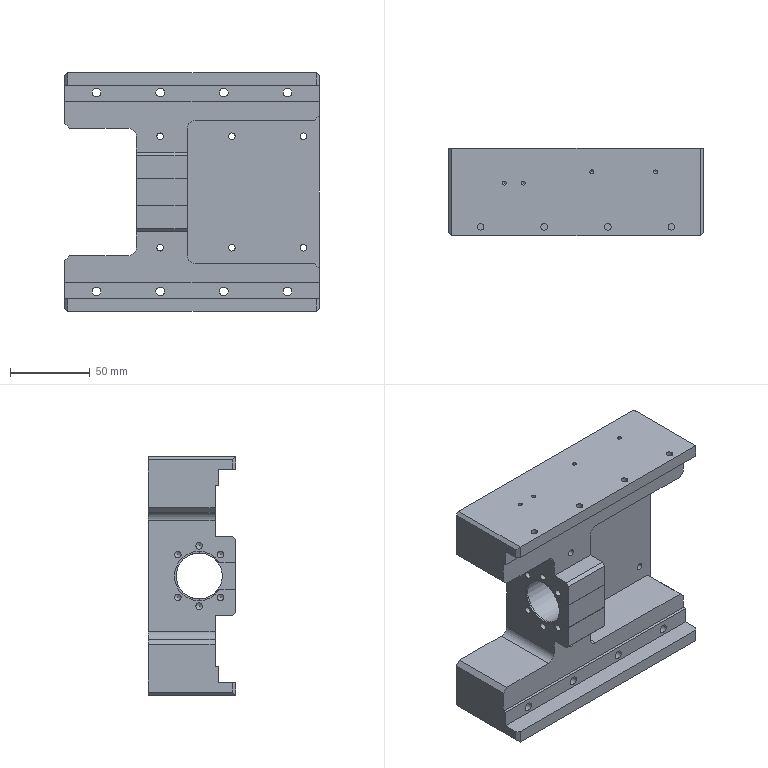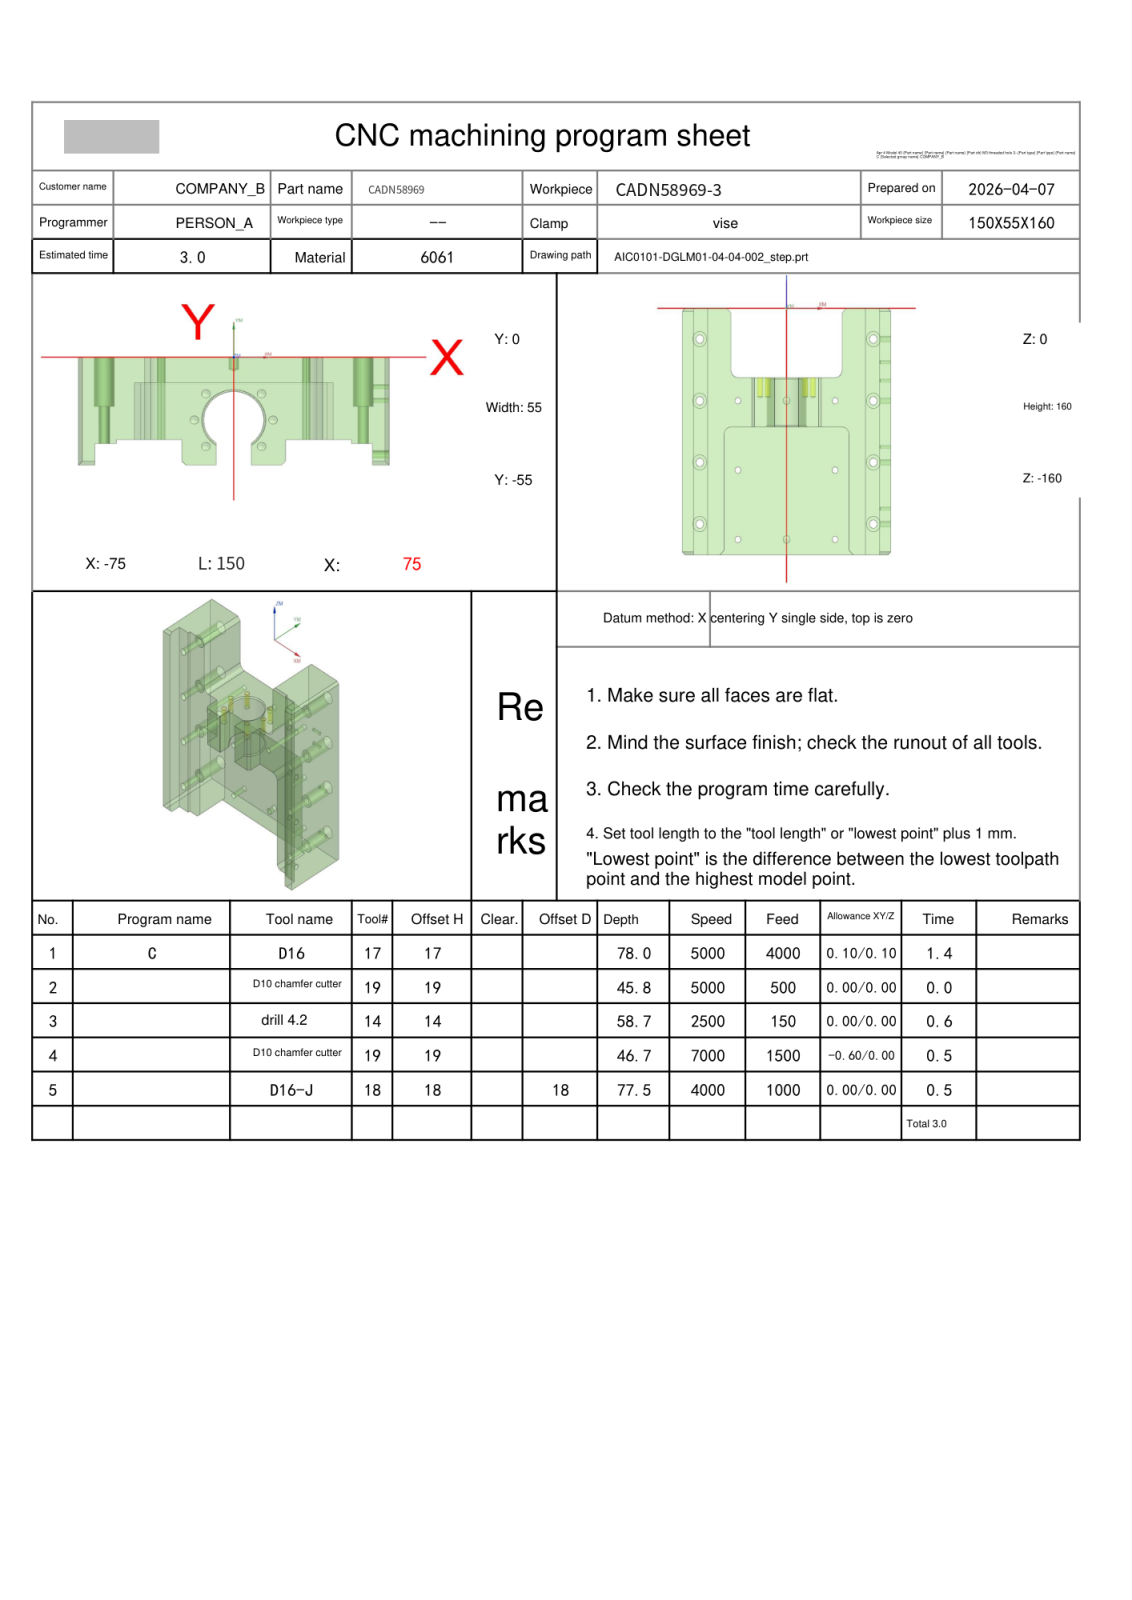NC program | NX | posted by the shop | part box 160 x 55 x 150 mm
Whole program:
%
O0001
(Machine time: 3.92 MIN)
(===Total Tool:4===)
(T17=D16    D=16.  R=0.   D-  H17 Z=-78.  )
(T19=D10 chamfer cutter D=10. R=0. D-H19 Z=-46.7 )
(T14=drill 4.2 D=4.2 DR_a=118 D-H14 Z=-58.66)
(T18=D16-J  D=16.  R=0.   D18 H18 Z=-77.5 )
G80 G90 G17 G49 G40
G91 G28 Z0
M01
N1 T17 M06
(D16  D=16. R=0. H=17 ce=0.10 di=0.10)
G00 G90 G54 X.4 Y-68.796 M03 S5000
G43 H17 Z20.
M08
Z-45.6
G01 Y-54.8 F4000.
Y-44.285
G02 X3.874 Y-37.538 I8.289 J-.001
G03 X6.759 Y-32. I-3.874 J5.538
X0.0 Y-25.241 I-6.759 J0.0
X-6.759 Y-32. I0.0 J-6.759
X-3.908 Y-37.514 I6.759 J0.0
G02 X-.4 Y-44.285 I-4.781 J-6.771
G01 Y-54.8
Y-68.796
G00 Z-46.2
G01 Y-54.8
Y-43.747
G03 X-3.752 Y-37.185 I-8.1 J0.0
G02 X-6.4 Y-32. I3.752 J5.185
X0.0 Y-25.6 I6.4 J0.0
X6.4 Y-32. I0.0 J-6.4
X3.752 Y-37.185 I-6.4 J0.0
G03 X.4 Y-43.747 I4.748 J-6.562
G01 Y-54.8
Y-68.796
G00 Z-46.8
G01 Y-54.8
Y-43.747
G02 X3.752 Y-37.185 I8.1 J0.0
G03 X6.4 Y-32. I-3.752 J5.185
X0.0 Y-25.6 I-6.4 J0.0
X-6.4 Y-32. I0.0 J-6.4
X-3.752 Y-37.185 I6.4 J0.0
G02 X-.4 Y-43.747 I-4.748 J-6.562
G01 Y-54.8
Y-68.796
G00 Z-47.4
G01 Y-54.8
Y-43.747
G03 X-3.752 Y-37.185 I-8.1 J0.0
G02 X-6.4 Y-32. I3.752 J5.185
X0.0 Y-25.6 I6.4 J0.0
X6.4 Y-32. I0.0 J-6.4
X3.752 Y-37.185 I-6.4 J0.0
G03 X.4 Y-43.747 I4.748 J-6.562
G01 Y-54.8
Y-68.796
G00 Z-48.
G01 Y-54.8
Y-43.747
G02 X3.752 Y-37.185 I8.1 J0.0
G03 X6.4 Y-32. I-3.752 J5.185
X0.0 Y-25.6 I-6.4 J0.0
X-6.4 Y-32. I0.0 J-6.4
X-3.752 Y-37.185 I6.4 J0.0
G02 X-.4 Y-43.747 I-4.748 J-6.562
G01 Y-54.8
Y-68.796
G00 Z-48.6
G01 Y-54.8
Y-43.747
G03 X-3.752 Y-37.185 I-8.1 J0.0
G02 X-6.4 Y-32. I3.752 J5.185
X0.0 Y-25.6 I6.4 J0.0
X6.4 Y-32. I0.0 J-6.4
X3.752 Y-37.185 I-6.4 J0.0
G03 X.4 Y-43.747 I4.748 J-6.562
G01 Y-54.8
Y-68.796
G00 Z-49.2
G01 Y-54.8
Y-43.747
G02 X3.752 Y-37.185 I8.1 J0.0
G03 X6.4 Y-32. I-3.752 J5.185
X0.0 Y-25.6 I-6.4 J0.0
X-6.4 Y-32. I0.0 J-6.4
X-3.752 Y-37.185 I6.4 J0.0
G02 X-.4 Y-43.747 I-4.748 J-6.562
G01 Y-54.8
Y-68.796
G00 Z-49.8
G01 Y-54.8
Y-43.747
G03 X-3.752 Y-37.185 I-8.1 J0.0
G02 X-6.4 Y-32. I3.752 J5.185
X0.0 Y-25.6 I6.4 J0.0
X6.4 Y-32. I0.0 J-6.4
X3.752 Y-37.185 I-6.4 J0.0
G03 X.4 Y-43.747 I4.748 J-6.562
G01 Y-54.8
Y-68.796
G00 Z-50.4
G01 Y-54.8
Y-43.747
G02 X3.752 Y-37.185 I8.1 J0.0
G03 X6.4 Y-32. I-3.752 J5.185
X0.0 Y-25.6 I-6.4 J0.0
X-6.4 Y-32. I0.0 J-6.4
X-3.752 Y-37.185 I6.4 J0.0
G02 X-.4 Y-43.747 I-4.748 J-6.562
G01 Y-54.8
Y-68.796
G00 Z-51.
G01 Y-54.8
Y-43.747
G03 X-3.752 Y-37.185 I-8.1 J0.0
G02 X-6.4 Y-32. I3.752 J5.185
X0.0 Y-25.6 I6.4 J0.0
X6.4 Y-32. I0.0 J-6.4
X3.752 Y-37.185 I-6.4 J0.0
G03 X.4 Y-43.747 I4.748 J-6.562
G01 Y-54.8
Y-68.796
G00 Z-51.6
G01 Y-54.8
Y-43.747
G02 X3.752 Y-37.185 I8.1 J0.0
G03 X6.4 Y-32. I-3.752 J5.185
X0.0 Y-25.6 I-6.4 J0.0
X-6.4 Y-32. I0.0 J-6.4
X-3.752 Y-37.185 I6.4 J0.0
G02 X-.4 Y-43.747 I-4.748 J-6.562
G01 Y-54.8
Y-68.796
G00 Z-52.2
G01 Y-54.8
Y-43.747
G03 X-3.752 Y-37.185 I-8.1 J0.0
G02 X-6.4 Y-32. I3.752 J5.185
X0.0 Y-25.6 I6.4 J0.0
X6.4 Y-32. I0.0 J-6.4
X3.752 Y-37.185 I-6.4 J0.0
G03 X.4 Y-43.747 I4.748 J-6.562
G01 Y-54.8
Y-68.796
G00 Z-52.8
G01 Y-54.8
Y-43.747
G02 X3.752 Y-37.185 I8.1 J0.0
G03 X6.4 Y-32. I-3.752 J5.185
X0.0 Y-25.6 I-6.4 J0.0
X-6.4 Y-32. I0.0 J-6.4
X-3.752 Y-37.185 I6.4 J0.0
G02 X-.4 Y-43.747 I-4.748 J-6.562
G01 Y-54.8
Y-68.796
G00 Z-53.4
G01 Y-54.8
Y-43.747
G03 X-3.752 Y-37.185 I-8.1 J0.0
G02 X-6.4 Y-32. I3.752 J5.185
X0.0 Y-25.6 I6.4 J0.0
X6.4 Y-32. I0.0 J-6.4
X3.752 Y-37.185 I-6.4 J0.0
G03 X.4 Y-43.747 I4.748 J-6.562
G01 Y-54.8
Y-68.796
G00 Z-54.
G01 Y-54.8
Y-43.747
G02 X3.752 Y-37.185 I8.1 J0.0
G03 X6.4 Y-32. I-3.752 J5.185
X0.0 Y-25.6 I-6.4 J0.0
X-6.4 Y-32. I0.0 J-6.4
X-3.752 Y-37.185 I6.4 J0.0
G02 X-.4 Y-43.747 I-4.748 J-6.562
G01 Y-54.8
Y-68.796
G00 Z-54.6
G01 Y-54.8
Y-43.747
G03 X-3.752 Y-37.185 I-8.1 J0.0
G02 X-6.4 Y-32. I3.752 J5.185
X0.0 Y-25.6 I6.4 J0.0
X6.4 Y-32. I0.0 J-6.4
X3.752 Y-37.185 I-6.4 J0.0
G03 X.4 Y-43.747 I4.748 J-6.562
G01 Y-54.8
Y-68.796
G00 Z-55.2
G01 Y-54.8
Y-43.747
G02 X3.752 Y-37.185 I8.1 J0.0
G03 X6.4 Y-32. I-3.752 J5.185
X0.0 Y-25.6 I-6.4 J0.0
X-6.4 Y-32. I0.0 J-6.4
X-3.752 Y-37.185 I6.4 J0.0
G02 X-.4 Y-43.747 I-4.748 J-6.562
G01 Y-54.8
Y-68.796
G00 Z-55.8
G01 Y-54.8
Y-43.747
G03 X-3.752 Y-37.185 I-8.1 J0.0
G02 X-6.4 Y-32. I3.752 J5.185
X0.0 Y-25.6 I6.4 J0.0
X6.4 Y-32. I0.0 J-6.4
X3.752 Y-37.185 I-6.4 J0.0
G03 X.4 Y-43.747 I4.748 J-6.562
G01 Y-54.8
Y-68.796
G00 Z-56.4
G01 Y-54.8
Y-43.747
G02 X3.752 Y-37.185 I8.1 J0.0
G03 X6.4 Y-32. I-3.752 J5.185
X0.0 Y-25.6 I-6.4 J0.0
X-6.4 Y-32. I0.0 J-6.4
X-3.752 Y-37.185 I6.4 J0.0
G02 X-.4 Y-43.747 I-4.748 J-6.562
G01 Y-54.8
Y-68.796
G00 Z-57.
G01 Y-54.8
Y-43.747
G03 X-3.752 Y-37.185 I-8.1 J0.0
G02 X-6.4 Y-32. I3.752 J5.185
X0.0 Y-25.6 I6.4 J0.0
X6.4 Y-32. I0.0 J-6.4
X3.752 Y-37.185 I-6.4 J0.0
G03 X.4 Y-43.747 I4.748 J-6.562
G01 Y-54.8
Y-68.796
G00 Z-57.6
G01 Y-54.8
Y-43.747
G02 X3.752 Y-37.185 I8.1 J0.0
G03 X6.4 Y-32. I-3.752 J5.185
X0.0 Y-25.6 I-6.4 J0.0
X-6.4 Y-32. I0.0 J-6.4
X-3.752 Y-37.185 I6.4 J0.0
G02 X-.4 Y-43.747 I-4.748 J-6.562
G01 Y-54.8
Y-68.796
G00 Z-58.2
G01 Y-54.8
Y-43.747
G03 X-3.752 Y-37.185 I-8.1 J0.0
G02 X-6.4 Y-32. I3.752 J5.185
X0.0 Y-25.6 I6.4 J0.0
X6.4 Y-32. I0.0 J-6.4
X3.752 Y-37.185 I-6.4 J0.0
G03 X.4 Y-43.747 I4.748 J-6.562
G01 Y-54.8
Y-68.796
G00 Z-58.8
G01 Y-54.8
Y-43.747
G02 X3.752 Y-37.185 I8.1 J0.0
G03 X6.4 Y-32. I-3.752 J5.185
X0.0 Y-25.6 I-6.4 J0.0
X-6.4 Y-32. I0.0 J-6.4
X-3.752 Y-37.185 I6.4 J0.0
G02 X-.4 Y-43.747 I-4.748 J-6.562
G01 Y-54.8
Y-68.796
G00 Z-59.4
G01 Y-54.8
Y-43.747
G03 X-3.752 Y-37.185 I-8.1 J0.0
G02 X-6.4 Y-32. I3.752 J5.185
X0.0 Y-25.6 I6.4 J0.0
X6.4 Y-32. I0.0 J-6.4
X3.752 Y-37.185 I-6.4 J0.0
G03 X.4 Y-43.747 I4.748 J-6.562
G01 Y-54.8
Y-68.796
G00 Z-60.
G01 Y-54.8
Y-43.747
G02 X3.752 Y-37.185 I8.1 J0.0
G03 X6.4 Y-32. I-3.752 J5.185
X0.0 Y-25.6 I-6.4 J0.0
X-6.4 Y-32. I0.0 J-6.4
X-3.752 Y-37.185 I6.4 J0.0
G02 X-.4 Y-43.747 I-4.748 J-6.562
G01 Y-54.8
Y-68.796
G00 Z-60.6
G01 Y-54.8
Y-43.747
G03 X-3.752 Y-37.185 I-8.1 J0.0
G02 X-6.4 Y-32. I3.752 J5.185
X0.0 Y-25.6 I6.4 J0.0
X6.4 Y-32. I0.0 J-6.4
X3.752 Y-37.185 I-6.4 J0.0
G03 X.4 Y-43.747 I4.748 J-6.562
G01 Y-54.8
Y-68.796
G00 Z-61.2
G01 Y-54.8
Y-43.747
G02 X3.752 Y-37.185 I8.1 J0.0
G03 X6.4 Y-32. I-3.752 J5.185
X0.0 Y-25.6 I-6.4 J0.0
X-6.4 Y-32. I0.0 J-6.4
X-3.752 Y-37.185 I6.4 J0.0
G02 X-.4 Y-43.747 I-4.748 J-6.562
G01 Y-54.8
Y-68.796
G00 Z-61.8
G01 Y-54.8
Y-43.747
G03 X-3.752 Y-37.185 I-8.1 J0.0
G02 X-6.4 Y-32. I3.752 J5.185
X0.0 Y-25.6 I6.4 J0.0
X6.4 Y-32. I0.0 J-6.4
X3.752 Y-37.185 I-6.4 J0.0
G03 X.4 Y-43.747 I4.748 J-6.562
G01 Y-54.8
Y-68.796
G00 Z-62.4
G01 Y-54.8
Y-43.747
G02 X3.752 Y-37.185 I8.1 J0.0
G03 X6.4 Y-32. I-3.752 J5.185
X0.0 Y-25.6 I-6.4 J0.0
X-6.4 Y-32. I0.0 J-6.4
X-3.752 Y-37.185 I6.4 J0.0
G02 X-.4 Y-43.747 I-4.748 J-6.562
G01 Y-54.8
Y-68.796
G00 Z-63.
G01 Y-54.8
Y-43.747
G03 X-3.752 Y-37.185 I-8.1 J0.0
G02 X-6.4 Y-32. I3.752 J5.185
X0.0 Y-25.6 I6.4 J0.0
X6.4 Y-32. I0.0 J-6.4
X3.752 Y-37.185 I-6.4 J0.0
G03 X.4 Y-43.747 I4.748 J-6.562
G01 Y-54.8
Y-68.796
G00 Z-63.6
G01 Y-54.8
Y-43.747
G02 X3.752 Y-37.185 I8.1 J0.0
G03 X6.4 Y-32. I-3.752 J5.185
X0.0 Y-25.6 I-6.4 J0.0
X-6.4 Y-32. I0.0 J-6.4
X-3.752 Y-37.185 I6.4 J0.0
G02 X-.4 Y-43.747 I-4.748 J-6.562
G01 Y-54.8
Y-68.796
G00 Z-64.2
G01 Y-54.8
Y-43.747
G03 X-3.752 Y-37.185 I-8.1 J0.0
G02 X-6.4 Y-32. I3.752 J5.185
X0.0 Y-25.6 I6.4 J0.0
X6.4 Y-32. I0.0 J-6.4
X3.752 Y-37.185 I-6.4 J0.0
G03 X.4 Y-43.747 I4.748 J-6.562
G01 Y-54.8
Y-68.796
G00 Z-64.8
G01 Y-54.8
Y-43.747
G02 X3.752 Y-37.185 I8.1 J0.0
G03 X6.4 Y-32. I-3.752 J5.185
X0.0 Y-25.6 I-6.4 J0.0
X-6.4 Y-32. I0.0 J-6.4
X-3.752 Y-37.185 I6.4 J0.0
G02 X-.4 Y-43.747 I-4.748 J-6.562
G01 Y-54.8
Y-68.796
G00 Z-65.4
G01 Y-54.8
Y-43.747
G03 X-3.752 Y-37.185 I-8.1 J0.0
G02 X-6.4 Y-32. I3.752 J5.185
X0.0 Y-25.6 I6.4 J0.0
X6.4 Y-32. I0.0 J-6.4
X3.752 Y-37.185 I-6.4 J0.0
G03 X.4 Y-43.747 I4.748 J-6.562
G01 Y-54.8
Y-68.796
G00 Z-66.
G01 Y-54.8
Y-43.747
G02 X3.752 Y-37.185 I8.1 J0.0
G03 X6.4 Y-32. I-3.752 J5.185
X0.0 Y-25.6 I-6.4 J0.0
X-6.4 Y-32. I0.0 J-6.4
X-3.752 Y-37.185 I6.4 J0.0
G02 X-.4 Y-43.747 I-4.748 J-6.562
G01 Y-54.8
Y-68.796
G00 Z-66.6
G01 Y-54.8
Y-43.747
G03 X-3.752 Y-37.185 I-8.1 J0.0
G02 X-6.4 Y-32. I3.752 J5.185
X0.0 Y-25.6 I6.4 J0.0
X6.4 Y-32. I0.0 J-6.4
X3.752 Y-37.185 I-6.4 J0.0
G03 X.4 Y-43.747 I4.748 J-6.562
G01 Y-54.8
Y-68.796
G00 Z-67.2
G01 Y-54.8
Y-43.747
G02 X3.752 Y-37.185 I8.1 J0.0
G03 X6.4 Y-32. I-3.752 J5.185
X0.0 Y-25.6 I-6.4 J0.0
X-6.4 Y-32. I0.0 J-6.4
X-3.752 Y-37.185 I6.4 J0.0
G02 X-.4 Y-43.747 I-4.748 J-6.562
G01 Y-54.8
Y-68.796
G00 Z-67.8
G01 Y-54.8
Y-43.747
G03 X-3.752 Y-37.185 I-8.1 J0.0
G02 X-6.4 Y-32. I3.752 J5.185
X0.0 Y-25.6 I6.4 J0.0
X6.4 Y-32. I0.0 J-6.4
X3.752 Y-37.185 I-6.4 J0.0
G03 X.4 Y-43.747 I4.748 J-6.562
G01 Y-54.8
Y-68.796
G00 Z-68.4
G01 Y-54.8
Y-43.747
G02 X3.752 Y-37.185 I8.1 J0.0
G03 X6.4 Y-32. I-3.752 J5.185
X0.0 Y-25.6 I-6.4 J0.0
X-6.4 Y-32. I0.0 J-6.4
X-3.752 Y-37.185 I6.4 J0.0
G02 X-.4 Y-43.747 I-4.748 J-6.562
G01 Y-54.8
Y-68.796
G00 Z-69.
G01 Y-54.8
Y-43.747
G03 X-3.752 Y-37.185 I-8.1 J0.0
G02 X-6.4 Y-32. I3.752 J5.185
X0.0 Y-25.6 I6.4 J0.0
X6.4 Y-32. I0.0 J-6.4
X3.752 Y-37.185 I-6.4 J0.0
G03 X.4 Y-43.747 I4.748 J-6.562
G01 Y-54.8
Y-68.796
G00 Z-69.6
G01 Y-54.8
Y-43.747
G02 X3.752 Y-37.185 I8.1 J0.0
G03 X6.4 Y-32. I-3.752 J5.185
X0.0 Y-25.6 I-6.4 J0.0
X-6.4 Y-32. I0.0 J-6.4
X-3.752 Y-37.185 I6.4 J0.0
G02 X-.4 Y-43.747 I-4.748 J-6.562
G01 Y-54.8
Y-68.796
G00 Z-70.2
G01 Y-54.8
Y-43.747
G03 X-3.752 Y-37.185 I-8.1 J0.0
G02 X-6.4 Y-32. I3.752 J5.185
X0.0 Y-25.6 I6.4 J0.0
X6.4 Y-32. I0.0 J-6.4
X3.752 Y-37.185 I-6.4 J0.0
G03 X.4 Y-43.747 I4.748 J-6.562
G01 Y-54.8
Y-68.796
G00 Z-70.8
G01 Y-54.8
Y-43.747
G02 X3.752 Y-37.185 I8.1 J0.0
G03 X6.4 Y-32. I-3.752 J5.185
X0.0 Y-25.6 I-6.4 J0.0
X-6.4 Y-32. I0.0 J-6.4
X-3.752 Y-37.185 I6.4 J0.0
G02 X-.4 Y-43.747 I-4.748 J-6.562
G01 Y-54.8
Y-68.796
G00 Z-71.4
G01 Y-54.8
Y-43.747
G03 X-3.752 Y-37.185 I-8.1 J0.0
G02 X-6.4 Y-32. I3.752 J5.185
X0.0 Y-25.6 I6.4 J0.0
X6.4 Y-32. I0.0 J-6.4
X3.752 Y-37.185 I-6.4 J0.0
G03 X.4 Y-43.747 I4.748 J-6.562
G01 Y-54.8
Y-68.796
G00 Z-72.
G01 Y-54.8
Y-43.747
G02 X3.752 Y-37.185 I8.1 J0.0
G03 X6.4 Y-32. I-3.752 J5.185
X0.0 Y-25.6 I-6.4 J0.0
X-6.4 Y-32. I0.0 J-6.4
X-3.752 Y-37.185 I6.4 J0.0
G02 X-.4 Y-43.747 I-4.748 J-6.562
G01 Y-54.8
Y-68.796
G00 Z-72.6
G01 Y-54.8
Y-43.747
G03 X-3.752 Y-37.185 I-8.1 J0.0
G02 X-6.4 Y-32. I3.752 J5.185
X0.0 Y-25.6 I6.4 J0.0
X6.4 Y-32. I0.0 J-6.4
X3.752 Y-37.185 I-6.4 J0.0
G03 X.4 Y-43.747 I4.748 J-6.562
G01 Y-54.8
Y-68.796
G00 Z-73.2
G01 Y-54.8
Y-43.747
G02 X3.752 Y-37.185 I8.1 J0.0
G03 X6.4 Y-32. I-3.752 J5.185
X0.0 Y-25.6 I-6.4 J0.0
X-6.4 Y-32. I0.0 J-6.4
X-3.752 Y-37.185 I6.4 J0.0
G02 X-.4 Y-43.747 I-4.748 J-6.562
G01 Y-54.8
Y-68.796
G00 Z-73.8
G01 Y-54.8
Y-43.747
G03 X-3.752 Y-37.185 I-8.1 J0.0
G02 X-6.4 Y-32. I3.752 J5.185
X0.0 Y-25.6 I6.4 J0.0
X6.4 Y-32. I0.0 J-6.4
X3.752 Y-37.185 I-6.4 J0.0
G03 X.4 Y-43.747 I4.748 J-6.562
G01 Y-54.8
Y-68.796
G00 Z-74.4
G01 Y-54.8
Y-43.747
G02 X3.752 Y-37.185 I8.1 J0.0
G03 X6.4 Y-32. I-3.752 J5.185
X0.0 Y-25.6 I-6.4 J0.0
X-6.4 Y-32. I0.0 J-6.4
X-3.752 Y-37.185 I6.4 J0.0
G02 X-.4 Y-43.747 I-4.748 J-6.562
G01 Y-54.8
Y-68.796
G00 Z-75.
G01 Y-54.8
Y-43.747
G03 X-3.752 Y-37.185 I-8.1 J0.0
G02 X-6.4 Y-32. I3.752 J5.185
X0.0 Y-25.6 I6.4 J0.0
X6.4 Y-32. I0.0 J-6.4
X3.752 Y-37.185 I-6.4 J0.0
G03 X.4 Y-43.747 I4.748 J-6.562
G01 Y-54.8
Y-68.796
G00 Z-75.6
G01 Y-54.8
Y-43.747
G02 X3.752 Y-37.185 I8.1 J0.0
G03 X6.4 Y-32. I-3.752 J5.185
X0.0 Y-25.6 I-6.4 J0.0
X-6.4 Y-32. I0.0 J-6.4
X-3.752 Y-37.185 I6.4 J0.0
G02 X-.4 Y-43.747 I-4.748 J-6.562
G01 Y-54.8
Y-68.796
G00 Z-76.2
G01 Y-54.8
Y-43.747
G03 X-3.752 Y-37.185 I-8.1 J0.0
G02 X-6.4 Y-32. I3.752 J5.185
X0.0 Y-25.6 I6.4 J0.0
X6.4 Y-32. I0.0 J-6.4
X3.752 Y-37.185 I-6.4 J0.0
G03 X.4 Y-43.747 I4.748 J-6.562
G01 Y-54.8
Y-68.796
G00 Z-76.8
G01 Y-54.8
Y-43.747
G02 X3.752 Y-37.185 I8.1 J0.0
G03 X6.4 Y-32. I-3.752 J5.185
X0.0 Y-25.6 I-6.4 J0.0
X-6.4 Y-32. I0.0 J-6.4
X-3.752 Y-37.185 I6.4 J0.0
G02 X-.4 Y-43.747 I-4.748 J-6.562
G01 Y-54.8
Y-68.796
G00 Z-77.4
G01 Y-54.8
Y-43.747
G03 X-3.752 Y-37.185 I-8.1 J0.0
G02 X-6.4 Y-32. I3.752 J5.185
X0.0 Y-25.6 I6.4 J0.0
X6.4 Y-32. I0.0 J-6.4
X3.752 Y-37.185 I-6.4 J0.0
G03 X.4 Y-43.747 I4.748 J-6.562
G01 Y-54.8
Y-68.796
G00 Z-78.
G01 Y-54.8
Y-43.747
G02 X3.752 Y-37.185 I8.1 J0.0
G03 X6.4 Y-32. I-3.752 J5.185
X0.0 Y-25.6 I-6.4 J0.0
X-6.4 Y-32. I0.0 J-6.4
X-3.752 Y-37.185 I6.4 J0.0
G02 X-.4 Y-43.747 I-4.748 J-6.562
G01 Y-54.8
Y-68.796
G00 Z20.
G91 G28 Z0.0
M05
M09
G91 G28 Z0.0
M01
N2 T19 M06
(D10 chamfer cutter D=10. R=0. H=19 ce=0.00 di=0.10)
G00 G90 G54 X-13.435 Y-18.565 M03 S5000
G43 H19 Z20.
M08
G98 G81 X-13.435 Y-18.565 Z-45.8 R-44. F500.
X-19. Y-32.
X-13.435 Y-45.435
X13.435
X19. Y-32.
X13.435 Y-18.565
G80
G00 Z20.
G91 G28 Z0.0
M05
M09
G91 G28 Z0.0
M01
N3 T14 M06
(drill 4.2 D=4.2 DR_a=118 H=14)
G00 G90 G54 X-13.435 Y-18.565 M03 S2500
G43 H14 Z20.
M08
G98 G83 X-13.435 Y-18.565 Z-58.662 R-44. F150. Q3.
X-19. Y-32.
X-13.435 Y-45.435
X13.435
X19. Y-32.
X13.435 Y-18.565
G80
G00 Z20.
G91 G28 Z0.0
M05
M09
G91 G28 Z0.0
M01
N4 T19 M06
(D10 chamfer cutter D=10. R=0. H=19 ce=-0.60 di=0.00)
G00 G90 G54 X13.832 Y-18.815 M03 S5000
G43 H19 Z20.
M08
Z-45.7
G01 Z-46.2 F500.
G03 X12.582 Y-18.48 I-1.25 J-2.165
X11.935 Y-18.565 I0.0 J-2.5
X13.435 Y-20.065 I1.5 J0.0
X14.935 Y-18.565 I0.0 J1.5
X13.435 Y-17.065 I-1.5 J0.0
X11.935 Y-18.565 I0.0 J-1.5
X12.582 Y-18.65 I.647 J2.415
X13.832 Y-18.315 I0.0 J2.5
G01 Z-45.7
G00 Z20.
X19.397 Y-32.25
Z-45.7
G01 Z-46.2
G03 X18.147 Y-31.915 I-1.25 J-2.165
X17.5 Y-32. I0.0 J-2.5
X19. Y-33.5 I1.5 J0.0
X20.5 Y-32. I0.0 J1.5
X19. Y-30.5 I-1.5 J0.0
X17.5 Y-32. I0.0 J-1.5
X18.147 Y-32.085 I.647 J2.415
X19.397 Y-31.75 I0.0 J2.5
G01 Z-45.7
G00 Z20.
X13.832 Y-45.685
Z-45.7
G01 Z-46.2
G03 X12.582 Y-45.35 I-1.25 J-2.165
X11.935 Y-45.435 I0.0 J-2.5
X13.435 Y-46.935 I1.5 J0.0
X14.935 Y-45.435 I0.0 J1.5
X13.435 Y-43.935 I-1.5 J0.0
X11.935 Y-45.435 I0.0 J-1.5
X12.582 Y-45.52 I.647 J2.415
X13.832 Y-45.185 I0.0 J2.5
G01 Z-45.7
G00 Z20.
X-13.038 Y-45.685
Z-45.7
G01 Z-46.2
G03 X-14.288 Y-45.35 I-1.25 J-2.165
X-14.935 Y-45.435 I0.0 J-2.5
X-13.435 Y-46.935 I1.5 J0.0
X-11.935 Y-45.435 I0.0 J1.5
X-13.435 Y-43.935 I-1.5 J0.0
X-14.935 Y-45.435 I0.0 J-1.5
X-14.288 Y-45.52 I.647 J2.415
X-13.038 Y-45.185 I0.0 J2.5
G01 Z-45.7
G00 Z20.
X-18.603 Y-32.25
Z-45.7
G01 Z-46.2
G03 X-19.853 Y-31.915 I-1.25 J-2.165
X-20.5 Y-32. I0.0 J-2.5
X-19. Y-33.5 I1.5 J0.0
X-17.5 Y-32. I0.0 J1.5
X-19. Y-30.5 I-1.5 J0.0
X-20.5 Y-32. I0.0 J-1.5
X-19.853 Y-32.085 I.647 J2.415
X-18.603 Y-31.75 I0.0 J2.5
G01 Z-45.7
G00 Z20.
X-13.038 Y-18.815
Z-45.7
G01 Z-46.2
G03 X-14.288 Y-18.48 I-1.25 J-2.165
X-14.935 Y-18.565 I0.0 J-2.5
X-13.435 Y-20.065 I1.5 J0.0
X-11.935 Y-18.565 I0.0 J1.5
X-13.435 Y-17.065 I-1.5 J0.0
X-14.935 Y-18.565 I0.0 J-1.5
X-14.288 Y-18.65 I.647 J2.415
X-13.038 Y-18.315 I0.0 J2.5
G01 Z-45.7
G00 Z20.
G00 G90 X10.823 Y-27.298 M03 S5000
Z20.
Z-45.2
G01 Z-46.7 F600.
X10.965 Y-27.204
G03 X11.869 Y-25.531 I-1.096 J1.673
X11.542 Y-24.435 I-2. J0.0
X11.388 Y-24.205 I-11.542 J-7.565
X11.165 Y-23.89 I-11.388 J-7.795
X10.863 Y-23.49 I-11.165 J-8.11
X10.693 Y-23.277 I-10.863 J-8.51
X7.752 Y-20.583 I-10.693 J-8.723
X7.211 Y-20.234 I-7.752 J-11.417
X4.695 Y-19.023 I-7.211 J-11.766
X4.496 Y-18.953 I-4.695 J-12.977
X2.926 Y-18.514 I-4.496 J-13.047
X2.537 Y-18.435 I-2.926 J-13.486
X.275 Y-18.203 I-2.537 J-13.565
G01 X.145 Y-18.201
X0.0 Y-18.2
G03 X-.271 Y-18.203 I0.0 J-13.8
X-.566 Y-18.212 I.271 J-13.797
G01 X-.687 Y-18.217
X-.769 Y-18.221
X-.939 Y-18.232
G03 X-2.013 Y-18.348 I.939 J-13.768
X-11.178 Y-23.907 I2.013 J-13.652
G01 X-11.239 Y-23.992
X-11.283 Y-24.054
X-11.357 Y-24.161
G03 X-11.559 Y-24.461 I11.357 J-7.839
X-11.697 Y-24.678 I11.559 J-7.539
X-11.947 Y-25.094 I11.697 J-7.322
G01 X-12.025 Y-25.23
G03 X-12.152 Y-25.461 I12.025 J-6.77
X-12.408 Y-25.96 I12.152 J-6.539
X-13.8 Y-32. I12.408 J-6.04
X-13.556 Y-34.582 I13.8 J0.0
X-13.365 Y-35.439 I13.556 J2.582
X-10.359 Y-41.117 I13.365 J3.439
X-9.732 Y-41.784 I10.359 J9.117
G01 X-9.634 Y-41.88
G03 X-9.063 Y-42.407 I9.634 J9.88
X-8.484 Y-42.884 I9.063 J10.407
G01 X-8.411 Y-42.941
G03 X-8.23 Y-43.077 I8.411 J10.941
X-8.026 Y-43.226 I8.23 J11.077
G01 X-7.973 Y-43.263
G03 X-7.631 Y-43.498 I7.973 J11.263
G01 X-7.568 Y-43.54
X0.0 Y-48.503
X7.572 Y-43.537
X7.631 Y-43.498
G03 X8.034 Y-43.22 I-7.631 J11.498
G01 X8.139 Y-43.144
X8.19 Y-43.107
G03 X8.357 Y-42.982 I-8.19 J11.107
G01 X8.434 Y-42.923
G03 X8.714 Y-42.701 I-8.434 J10.923
X9.016 Y-42.447 I-8.714 J10.701
X9.388 Y-42.114 I-9.016 J10.447
G01 X9.479 Y-42.03
X9.561 Y-41.952
G03 X9.767 Y-41.749 I-9.561 J9.951
X10.494 Y-40.962 I-9.767 J9.749
X10.743 Y-40.662 I-10.494 J8.962
X11.143 Y-40.14 I-10.743 J8.662
X11.348 Y-39.852 I-11.143 J8.14
G01 X11.383 Y-39.802
G03 X11.51 Y-39.614 I-11.383 J7.802
G01 X11.578 Y-39.51
G03 X11.967 Y-38.873 I-11.578 J7.51
X12.105 Y-38.626 I-11.967 J6.873
G01 X12.196 Y-38.458
G03 X12.956 Y-36.752 I-12.196 J6.458
X13.8 Y-32. I-12.956 J4.752
X13.632 Y-29.855 I-13.8 J0.0
X13.576 Y-29.524 I-13.632 J-2.145
X13.422 Y-28.793 I-13.576 J-2.476
X11.542 Y-24.435 I-13.422 J-3.207
X11.388 Y-24.205 I-11.542 J-7.565
G01 X11.318 Y-24.104
G03 X9.677 Y-23.248 I-1.64 J-1.144
X8.533 Y-23.608 I0.0 J-2.
G01 X8.393 Y-23.706
Z-45.2
G00 Z20.
G00 G90 X7.8 Y-46.005 M03 S7000
Z20.
Z-42.5
G01 Y-54.753 Z-45.684 F1500.
X7.838 Y-54.96 Z-45.761
X7.919 Y-55.155 Z-45.837
X8.038 Y-55.328 Z-45.914
X8.205 Y-55.495 Z-46.
X8.093 Y-55.383
G02 X7.8 Y-54.676 I.707 J.707
G01 Y-44.961
Z-43.5
G00 Z20.
X-7.8 Y-54.578
Z-42.5
G01 Y-44.961 Z-46.
Y-54.676
G02 X-8.093 Y-55.383 I-1. J0.0
G01 X-8.205 Y-55.495
Z-43.5
G00 Z20.
G91 G28 Z0.0
M05
M09
G91 G28 Z0.0
M01
N5 T18 M06
(D16-J  D=16. R=0. H=18 ce=0.00 di=0.00)
G00 G90 G54 X8.559 Y-69.849 M03 S4000
G43 H18 Z10.
M08
Z-51.625
G01 Z-53.125 F1000.
G41 D18
X8.7 Y-69.708
G03 X9.403 Y-68.011 I-1.697 J1.697
X8.7 Y-66.314 I-2.4 J0.0
G01 X.5 Y-58.114
Y-39.661
X3.81 Y-37.266
G03 X6.5 Y-32. I-3.81 J5.266
X0.0 Y-25.5 I-6.5 J0.0
X-6.5 Y-32. I0.0 J-6.5
X-3.81 Y-37.266 I6.5 J0.0
G01 X-.5 Y-39.661
Y-58.114
X-8.7 Y-66.314
G03 X-9.403 Y-68.011 I1.697 J-1.697
X-8.7 Y-69.708 I2.4 J0.0
G01 G40 X-8.559 Y-69.849
Z-51.625
G00 X8.559
Z-59.75
G01 Z-61.25
G41 D18
X8.7 Y-69.708
G03 X9.403 Y-68.011 I-1.697 J1.697
X8.7 Y-66.314 I-2.4 J0.0
G01 X.5 Y-58.114
Y-39.661
X3.81 Y-37.266
G03 X6.5 Y-32. I-3.81 J5.266
X0.0 Y-25.5 I-6.5 J0.0
X-6.5 Y-32. I0.0 J-6.5
X-3.81 Y-37.266 I6.5 J0.0
G01 X-.5 Y-39.661
Y-58.114
X-8.7 Y-66.314
G03 X-9.403 Y-68.011 I1.697 J-1.697
X-8.7 Y-69.708 I2.4 J0.0
G01 G40 X-8.559 Y-69.849
Z-59.75
G00 X8.559
Z-67.875
G01 Z-69.375
G41 D18
X8.7 Y-69.708
G03 X9.403 Y-68.011 I-1.697 J1.697
X8.7 Y-66.314 I-2.4 J0.0
G01 X.5 Y-58.114
Y-39.661
X3.81 Y-37.266
G03 X6.5 Y-32. I-3.81 J5.266
X0.0 Y-25.5 I-6.5 J0.0
X-6.5 Y-32. I0.0 J-6.5
X-3.81 Y-37.266 I6.5 J0.0
G01 X-.5 Y-39.661
Y-58.114
X-8.7 Y-66.314
G03 X-9.403 Y-68.011 I1.697 J-1.697
X-8.7 Y-69.708 I2.4 J0.0
G01 G40 X-8.559 Y-69.849
Z-67.875
G00 X8.559
Z-76.
G01 Z-77.5
G41 D18
X8.7 Y-69.708
G03 X9.403 Y-68.011 I-1.697 J1.697
X8.7 Y-66.314 I-2.4 J0.0
G01 X.5 Y-58.114
Y-39.661
X3.81 Y-37.266
G03 X6.5 Y-32. I-3.81 J5.266
X0.0 Y-25.5 I-6.5 J0.0
X-6.5 Y-32. I0.0 J-6.5
X-3.81 Y-37.266 I6.5 J0.0
G01 X-.5 Y-39.661
Y-58.114
X-8.7 Y-66.314
G03 X-9.403 Y-68.011 I1.697 J-1.697
X-8.7 Y-69.708 I2.4 J0.0
G01 G40 X-8.559 Y-69.849
Z-76.
G00 Z10.
M05
M09
G91 G28 Z0.0
G91 G28 Y0.0
M30
%